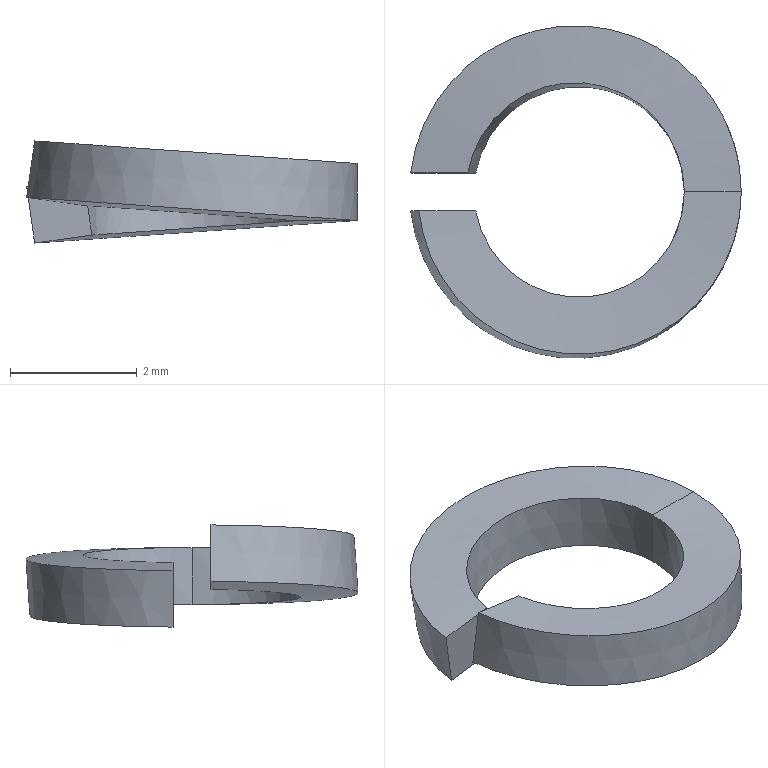Part | NX | features BREP 1 | 1 solid | 10 faces | box 5.22 x 5.25 x 1.612 mm | volume 10.428 mm3 | cone 8 | plane 2
STEP:
#1=CARTESIAN_POINT('',(-1.72,-0.3,0.2391));
#2=VERTEX_POINT('',#1);
#3=CARTESIAN_POINT('',(-2.62,-0.3,0.365));
#4=VERTEX_POINT('',#3);
#5=CARTESIAN_POINT('',(-1.72,-0.3,0.2391));
#6=CARTESIAN_POINT('',(-2.02,-0.3,0.281));
#7=CARTESIAN_POINT('',(-2.32,-0.3,0.323));
#8=CARTESIAN_POINT('',(-2.62,-0.3,0.365));
#9=B_SPLINE_CURVE_WITH_KNOTS('',3,(#5,#6,#7,#8),.UNSPECIFIED.,.F.,.F.,(4,4),(0.,1.),.PIECEWISE_BEZIER_KNOTS.);
#10=EDGE_CURVE('',#2,#4,#9,.T.);
#11=ORIENTED_EDGE('',*,*,#10,.F.);
#12=CARTESIAN_POINT('',(1.7,0.,0.));
#13=VERTEX_POINT('',#12);
#14=CARTESIAN_POINT('',(-0.02304,0.,0.1205));
#15=DIRECTION('',(0.06976,0.,0.9976));
#16=DIRECTION('',(0.9976,0.,-0.06976));
#17=AXIS2_PLACEMENT_3D('',#14,#15,#16);
#18=CIRCLE('',#17,1.727);
#19=EDGE_CURVE('',#2,#13,#18,.T.);
#20=ORIENTED_EDGE('',*,*,#19,.T.);
#21=CARTESIAN_POINT('',(2.6,0.,0.));
#22=VERTEX_POINT('',#21);
#23=CARTESIAN_POINT('',(2.6,0.,0.));
#24=DIRECTION('',(-1.,0.,0.));
#25=VECTOR('',#24,1000.);
#26=LINE('',#23,#25);
#27=EDGE_CURVE('',#22,#13,#26,.T.);
#28=ORIENTED_EDGE('',*,*,#27,.F.);
#29=CARTESIAN_POINT('',(-0.01866,0.,0.1831));
#30=DIRECTION('',(0.06976,0.,0.9976));
#31=DIRECTION('',(0.9976,0.,-0.06976));
#32=AXIS2_PLACEMENT_3D('',#29,#30,#31);
#33=CIRCLE('',#32,2.625);
#34=EDGE_CURVE('',#4,#22,#33,.T.);
#35=ORIENTED_EDGE('',*,*,#34,.F.);
#36=EDGE_LOOP('',(#11,#20,#28,#35));
#37=FACE_BOUND('',#36,.T.);
#38=CARTESIAN_POINT('',(-0.01866,0.,0.1831));
#39=DIRECTION('',(0.06976,0.,0.9976));
#40=DIRECTION('',(-0.9976,0.,0.06976));
#41=AXIS2_PLACEMENT_3D('',#38,#39,#40);
#42=CONICAL_SURFACE('',#41,2.625,1.501);
#43=ADVANCED_FACE('',(#37),#42,.T.);
#44=CARTESIAN_POINT('',(-1.594,-0.3,1.13));
#45=VERTEX_POINT('',#44);
#46=CARTESIAN_POINT('',(-1.594,-0.3,1.13));
#47=CARTESIAN_POINT('',(-1.613,-0.3,0.9951));
#48=CARTESIAN_POINT('',(-1.632,-0.3,0.8599));
#49=CARTESIAN_POINT('',(-1.671,-0.3,0.5861));
#50=CARTESIAN_POINT('',(-1.69,-0.3,0.4475));
#51=CARTESIAN_POINT('',(-1.713,-0.3,0.2857));
#52=CARTESIAN_POINT('',(-1.717,-0.3,0.2624));
#53=CARTESIAN_POINT('',(-1.72,-0.3,0.2391));
#54=B_SPLINE_CURVE_WITH_KNOTS('',3,(#46,#47,#48,#49,#50,#51,#52,#53),.UNSPECIFIED.,.F.,.F.,(4,2,2,4),(0.,0.4552,0.9217,1.),.UNSPECIFIED.);
#55=EDGE_CURVE('',#45,#2,#54,.T.);
#56=ORIENTED_EDGE('',*,*,#55,.F.);
#57=CARTESIAN_POINT('',(1.7,0.,0.9));
#58=VERTEX_POINT('',#57);
#59=CARTESIAN_POINT('',(0.03959,0.,1.016));
#60=DIRECTION('',(0.06976,0.,0.9976));
#61=DIRECTION('',(0.9976,0.,-0.06976));
#62=AXIS2_PLACEMENT_3D('',#59,#60,#61);
#63=CIRCLE('',#62,1.664);
#64=EDGE_CURVE('',#45,#58,#63,.T.);
#65=ORIENTED_EDGE('',*,*,#64,.T.);
#66=CARTESIAN_POINT('',(1.7,0.,0.));
#67=DIRECTION('',(0.,0.,1.));
#68=VECTOR('',#67,1000.);
#69=LINE('',#66,#68);
#70=EDGE_CURVE('',#13,#58,#69,.T.);
#71=ORIENTED_EDGE('',*,*,#70,.F.);
#72=ORIENTED_EDGE('',*,*,#19,.F.);
#73=EDGE_LOOP('',(#56,#65,#71,#72));
#74=FACE_BOUND('',#73,.T.);
#75=CARTESIAN_POINT('',(-0.02304,0.,0.1205));
#76=DIRECTION('',(-0.06976,0.,-0.9976));
#77=DIRECTION('',(0.9976,0.,-0.06976));
#78=AXIS2_PLACEMENT_3D('',#75,#76,#77);
#79=CONICAL_SURFACE('',#78,1.727,0.06981);
#80=ADVANCED_FACE('',(#74),#79,.F.);
#81=CARTESIAN_POINT('',(-2.494,-0.3,1.256));
#82=VERTEX_POINT('',#81);
#83=CARTESIAN_POINT('',(-2.494,-0.3,1.256));
#84=CARTESIAN_POINT('',(-2.194,-0.3,1.214));
#85=CARTESIAN_POINT('',(-1.894,-0.3,1.172));
#86=CARTESIAN_POINT('',(-1.594,-0.3,1.13));
#87=B_SPLINE_CURVE_WITH_KNOTS('',3,(#83,#84,#85,#86),.UNSPECIFIED.,.F.,.F.,(4,4),(0.,1.),.PIECEWISE_BEZIER_KNOTS.);
#88=EDGE_CURVE('',#82,#45,#87,.T.);
#89=ORIENTED_EDGE('',*,*,#88,.F.);
#90=CARTESIAN_POINT('',(2.6,0.,0.9));
#91=VERTEX_POINT('',#90);
#92=CARTESIAN_POINT('',(0.04397,0.,1.079));
#93=DIRECTION('',(0.06976,0.,0.9976));
#94=DIRECTION('',(0.9976,0.,-0.06976));
#95=AXIS2_PLACEMENT_3D('',#92,#93,#94);
#96=CIRCLE('',#95,2.562);
#97=EDGE_CURVE('',#82,#91,#96,.T.);
#98=ORIENTED_EDGE('',*,*,#97,.T.);
#99=CARTESIAN_POINT('',(1.7,0.,0.9));
#100=DIRECTION('',(1.,0.,0.));
#101=VECTOR('',#100,1000.);
#102=LINE('',#99,#101);
#103=EDGE_CURVE('',#58,#91,#102,.T.);
#104=ORIENTED_EDGE('',*,*,#103,.F.);
#105=ORIENTED_EDGE('',*,*,#64,.F.);
#106=EDGE_LOOP('',(#89,#98,#104,#105));
#107=FACE_BOUND('',#106,.T.);
#108=CARTESIAN_POINT('',(0.03959,0.,1.016));
#109=DIRECTION('',(0.06976,0.,0.9976));
#110=DIRECTION('',(-0.9976,0.,0.06976));
#111=AXIS2_PLACEMENT_3D('',#108,#109,#110);
#112=CONICAL_SURFACE('',#111,1.664,1.501);
#113=ADVANCED_FACE('',(#107),#112,.F.);
#114=CARTESIAN_POINT('',(-2.62,-0.3,0.365));
#115=CARTESIAN_POINT('',(-2.578,-0.3,0.6621));
#116=CARTESIAN_POINT('',(-2.536,-0.3,0.9592));
#117=CARTESIAN_POINT('',(-2.494,-0.3,1.256));
#118=B_SPLINE_CURVE_WITH_KNOTS('',3,(#114,#115,#116,#117),.UNSPECIFIED.,.F.,.F.,(4,4),(0.,1.),.PIECEWISE_BEZIER_KNOTS.);
#119=EDGE_CURVE('',#4,#82,#118,.T.);
#120=ORIENTED_EDGE('',*,*,#119,.F.);
#121=ORIENTED_EDGE('',*,*,#34,.T.);
#122=CARTESIAN_POINT('',(2.6,0.,0.9));
#123=DIRECTION('',(0.,0.,-1.));
#124=VECTOR('',#123,1000.);
#125=LINE('',#122,#124);
#126=EDGE_CURVE('',#91,#22,#125,.T.);
#127=ORIENTED_EDGE('',*,*,#126,.F.);
#128=ORIENTED_EDGE('',*,*,#97,.F.);
#129=EDGE_LOOP('',(#120,#121,#127,#128));
#130=FACE_BOUND('',#129,.T.);
#131=CARTESIAN_POINT('',(0.04397,0.,1.079));
#132=DIRECTION('',(-0.06976,0.,-0.9976));
#133=DIRECTION('',(0.9976,0.,-0.06976));
#134=AXIS2_PLACEMENT_3D('',#131,#132,#133);
#135=CONICAL_SURFACE('',#134,2.562,0.06981);
#136=ADVANCED_FACE('',(#130),#135,.T.);
#137=CARTESIAN_POINT('',(-1.594,0.3,-0.2303));
#138=VERTEX_POINT('',#137);
#139=CARTESIAN_POINT('',(0.03959,0.,-0.1161));
#140=DIRECTION('',(0.06976,0.,-0.9976));
#141=DIRECTION('',(-0.9976,0.,-0.06976));
#142=AXIS2_PLACEMENT_3D('',#139,#140,#141);
#143=CIRCLE('',#142,1.664);
#144=EDGE_CURVE('',#138,#13,#143,.T.);
#145=ORIENTED_EDGE('',*,*,#144,.F.);
#146=CARTESIAN_POINT('',(-2.494,0.3,-0.3562));
#147=VERTEX_POINT('',#146);
#148=CARTESIAN_POINT('',(-1.594,0.3,-0.2303));
#149=CARTESIAN_POINT('',(-1.894,0.3,-0.2722));
#150=CARTESIAN_POINT('',(-2.194,0.3,-0.3142));
#151=CARTESIAN_POINT('',(-2.494,0.3,-0.3562));
#152=B_SPLINE_CURVE_WITH_KNOTS('',3,(#148,#149,#150,#151),.UNSPECIFIED.,.F.,.F.,(4,4),(0.,1.),.PIECEWISE_BEZIER_KNOTS.);
#153=EDGE_CURVE('',#138,#147,#152,.T.);
#154=ORIENTED_EDGE('',*,*,#153,.T.);
#155=CARTESIAN_POINT('',(0.04397,0.,-0.1787));
#156=DIRECTION('',(0.06976,0.,-0.9976));
#157=DIRECTION('',(-0.9976,0.,-0.06976));
#158=AXIS2_PLACEMENT_3D('',#155,#156,#157);
#159=CIRCLE('',#158,2.562);
#160=EDGE_CURVE('',#147,#22,#159,.T.);
#161=ORIENTED_EDGE('',*,*,#160,.T.);
#162=ORIENTED_EDGE('',*,*,#27,.T.);
#163=EDGE_LOOP('',(#145,#154,#161,#162));
#164=FACE_BOUND('',#163,.T.);
#165=CARTESIAN_POINT('',(0.04397,0.,-0.1787));
#166=DIRECTION('',(0.06976,0.,-0.9976));
#167=DIRECTION('',(0.9976,0.,0.06976));
#168=AXIS2_PLACEMENT_3D('',#165,#166,#167);
#169=CONICAL_SURFACE('',#168,2.562,1.501);
#170=ADVANCED_FACE('',(#164),#169,.F.);
#171=CARTESIAN_POINT('',(-1.72,0.3,0.6609));
#172=VERTEX_POINT('',#171);
#173=CARTESIAN_POINT('',(-0.02304,0.,0.7795));
#174=DIRECTION('',(0.06976,0.,-0.9976));
#175=DIRECTION('',(-0.9976,0.,-0.06976));
#176=AXIS2_PLACEMENT_3D('',#173,#174,#175);
#177=CIRCLE('',#176,1.727);
#178=EDGE_CURVE('',#172,#58,#177,.T.);
#179=ORIENTED_EDGE('',*,*,#178,.F.);
#180=CARTESIAN_POINT('',(-1.72,0.3,0.6609));
#181=CARTESIAN_POINT('',(-1.69,0.3,0.4526));
#182=CARTESIAN_POINT('',(-1.661,0.3,0.2444));
#183=CARTESIAN_POINT('',(-1.619,0.3,-0.05267));
#184=CARTESIAN_POINT('',(-1.606,0.3,-0.1415));
#185=CARTESIAN_POINT('',(-1.594,0.3,-0.2303));
#186=B_SPLINE_CURVE_WITH_KNOTS('',3,(#180,#181,#182,#183,#184,#185),.UNSPECIFIED.,.F.,.F.,(4,2,4),(0.,0.701,1.),.UNSPECIFIED.);
#187=EDGE_CURVE('',#172,#138,#186,.T.);
#188=ORIENTED_EDGE('',*,*,#187,.T.);
#189=ORIENTED_EDGE('',*,*,#144,.T.);
#190=ORIENTED_EDGE('',*,*,#70,.T.);
#191=EDGE_LOOP('',(#179,#188,#189,#190));
#192=FACE_BOUND('',#191,.T.);
#193=CARTESIAN_POINT('',(0.03959,0.,-0.1161));
#194=DIRECTION('',(-0.06976,0.,0.9976));
#195=DIRECTION('',(-0.9976,0.,-0.06976));
#196=AXIS2_PLACEMENT_3D('',#193,#194,#195);
#197=CONICAL_SURFACE('',#196,1.664,0.06981);
#198=ADVANCED_FACE('',(#192),#197,.F.);
#199=CARTESIAN_POINT('',(-2.62,0.3,0.535));
#200=VERTEX_POINT('',#199);
#201=CARTESIAN_POINT('',(-0.01866,0.,0.7169));
#202=DIRECTION('',(0.06976,0.,-0.9976));
#203=DIRECTION('',(-0.9976,0.,-0.06976));
#204=AXIS2_PLACEMENT_3D('',#201,#202,#203);
#205=CIRCLE('',#204,2.625);
#206=EDGE_CURVE('',#200,#91,#205,.T.);
#207=ORIENTED_EDGE('',*,*,#206,.F.);
#208=CARTESIAN_POINT('',(-2.62,0.3,0.535));
#209=CARTESIAN_POINT('',(-2.32,0.3,0.577));
#210=CARTESIAN_POINT('',(-2.02,0.3,0.619));
#211=CARTESIAN_POINT('',(-1.72,0.3,0.6609));
#212=B_SPLINE_CURVE_WITH_KNOTS('',3,(#208,#209,#210,#211),.UNSPECIFIED.,.F.,.F.,(4,4),(0.,1.),.PIECEWISE_BEZIER_KNOTS.);
#213=EDGE_CURVE('',#200,#172,#212,.T.);
#214=ORIENTED_EDGE('',*,*,#213,.T.);
#215=ORIENTED_EDGE('',*,*,#178,.T.);
#216=ORIENTED_EDGE('',*,*,#103,.T.);
#217=EDGE_LOOP('',(#207,#214,#215,#216));
#218=FACE_BOUND('',#217,.T.);
#219=CARTESIAN_POINT('',(-0.02304,0.,0.7795));
#220=DIRECTION('',(0.06976,0.,-0.9976));
#221=DIRECTION('',(0.9976,0.,0.06976));
#222=AXIS2_PLACEMENT_3D('',#219,#220,#221);
#223=CONICAL_SURFACE('',#222,1.727,1.501);
#224=ADVANCED_FACE('',(#218),#223,.T.);
#225=ORIENTED_EDGE('',*,*,#160,.F.);
#226=CARTESIAN_POINT('',(-2.494,0.3,-0.3562));
#227=CARTESIAN_POINT('',(-2.508,0.3,-0.2625));
#228=CARTESIAN_POINT('',(-2.521,0.3,-0.1688));
#229=CARTESIAN_POINT('',(-2.563,0.3,0.1283));
#230=CARTESIAN_POINT('',(-2.591,0.3,0.3316));
#231=CARTESIAN_POINT('',(-2.62,0.3,0.535));
#232=B_SPLINE_CURVE_WITH_KNOTS('',3,(#226,#227,#228,#229,#230,#231),.UNSPECIFIED.,.F.,.F.,(4,2,4),(0.,0.3155,1.),.UNSPECIFIED.);
#233=EDGE_CURVE('',#147,#200,#232,.T.);
#234=ORIENTED_EDGE('',*,*,#233,.T.);
#235=ORIENTED_EDGE('',*,*,#206,.T.);
#236=ORIENTED_EDGE('',*,*,#126,.T.);
#237=EDGE_LOOP('',(#225,#234,#235,#236));
#238=FACE_BOUND('',#237,.T.);
#239=CARTESIAN_POINT('',(-0.01866,0.,0.7169));
#240=DIRECTION('',(-0.06976,0.,0.9976));
#241=DIRECTION('',(-0.9976,0.,-0.06976));
#242=AXIS2_PLACEMENT_3D('',#239,#240,#241);
#243=CONICAL_SURFACE('',#242,2.625,0.06981);
#244=ADVANCED_FACE('',(#238),#243,.T.);
#245=ORIENTED_EDGE('',*,*,#187,.F.);
#246=ORIENTED_EDGE('',*,*,#213,.F.);
#247=ORIENTED_EDGE('',*,*,#233,.F.);
#248=ORIENTED_EDGE('',*,*,#153,.F.);
#249=EDGE_LOOP('',(#245,#246,#247,#248));
#250=FACE_BOUND('',#249,.T.);
#251=CARTESIAN_POINT('',(0.,0.3,-5.2));
#252=DIRECTION('',(0.,1.,0.));
#253=DIRECTION('',(0.,0.,-1.));
#254=AXIS2_PLACEMENT_3D('',#251,#252,#253);
#255=PLANE('',#254);
#256=ADVANCED_FACE('',(#250),#255,.F.);
#257=ORIENTED_EDGE('',*,*,#10,.T.);
#258=ORIENTED_EDGE('',*,*,#119,.T.);
#259=ORIENTED_EDGE('',*,*,#88,.T.);
#260=ORIENTED_EDGE('',*,*,#55,.T.);
#261=EDGE_LOOP('',(#257,#258,#259,#260));
#262=FACE_BOUND('',#261,.T.);
#263=CARTESIAN_POINT('',(-5.2,-0.3,-5.2));
#264=DIRECTION('',(0.,-1.,0.));
#265=DIRECTION('',(0.,0.,1.));
#266=AXIS2_PLACEMENT_3D('',#263,#264,#265);
#267=PLANE('',#266);
#268=ADVANCED_FACE('',(#262),#267,.F.);
#269=CLOSED_SHELL('',(#43,#80,#113,#136,#170,#198,#224,#244,#256,#268));
#270=MANIFOLD_SOLID_BREP('',#269);
#271=(LENGTH_UNIT()NAMED_UNIT(*)SI_UNIT(.MILLI.,.METRE.));
#272=UNCERTAINTY_MEASURE_WITH_UNIT(LENGTH_MEASURE(0.00001),#271,'','');
#273=(NAMED_UNIT(*)PLANE_ANGLE_UNIT()SI_UNIT($,.RADIAN.));
#274=(NAMED_UNIT(*)SI_UNIT($,.STERADIAN.)SOLID_ANGLE_UNIT());
#275=(GEOMETRIC_REPRESENTATION_CONTEXT(3)GLOBAL_UNCERTAINTY_ASSIGNED_CONTEXT((#272))GLOBAL_UNIT_ASSIGNED_CONTEXT((#271,#273,#274))REPRESENTATION_CONTEXT('',''));
#276=ADVANCED_BREP_SHAPE_REPRESENTATION('',(#270),#275);